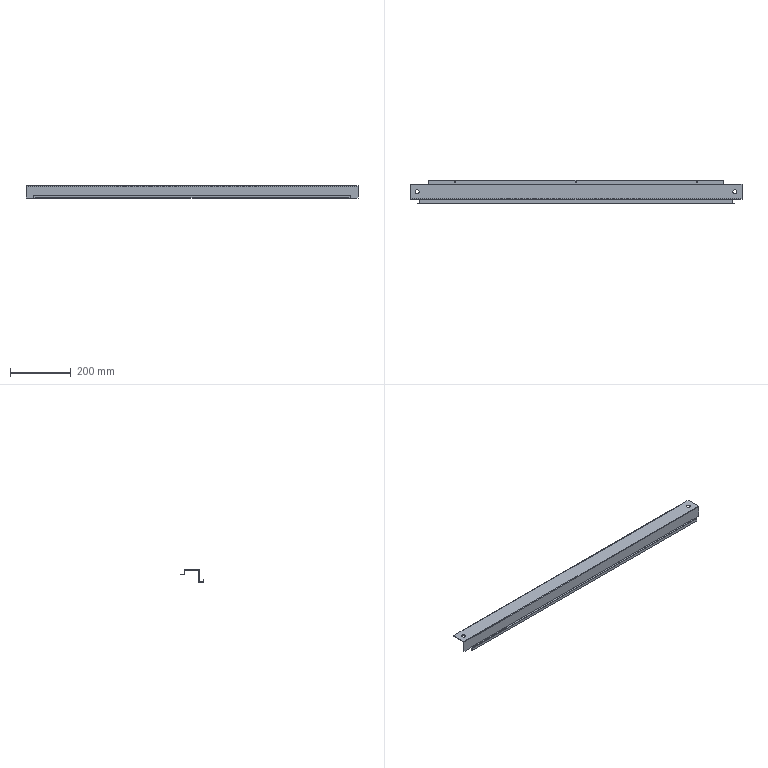Part | SolidWorks | features EdgeFlange 5, ICE 2, SMBaseFlange 2, FlatPattern 1, SheetMetal 1 | 1 solid | 88 faces | box 1097 x 78.5 x 40 mm | volume 218985 mm3 | plane 68 | cylinder 20 | commonest cylinder face diameters 5.1 x6 0.2 x5 3.2 x5 13 x4